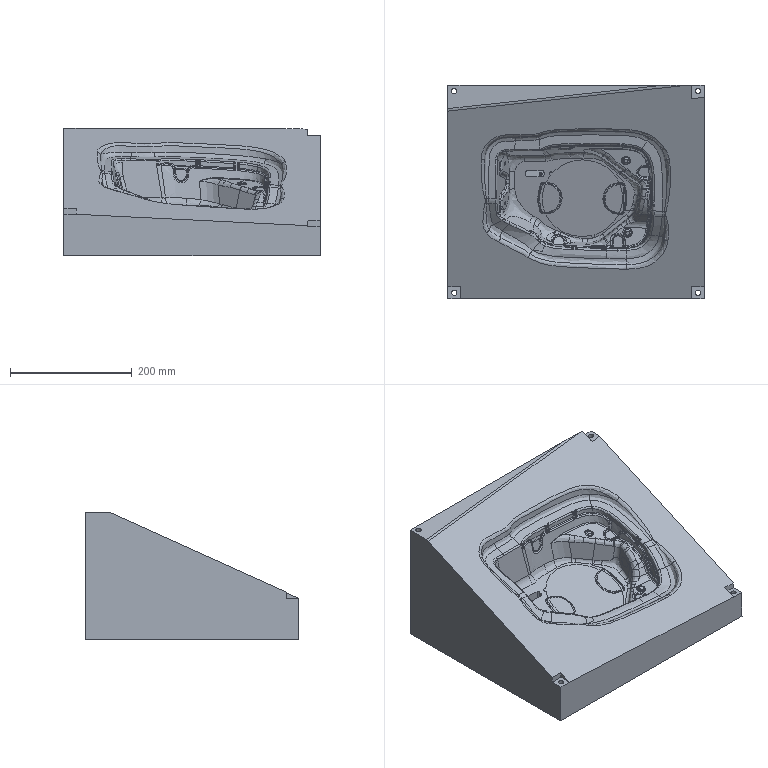Part | 1 solid | 714 faces | box 420 x 350 x 208.3 mm | volume 17507071 mm3 | spline 373 | cylinder 194 | plane 94 | sphere 44 | torus 7 | cone 2 | commonest cylinder face diameters 6 x31 4 x27 12 x10 10.3 x8 10 x7 20 x7